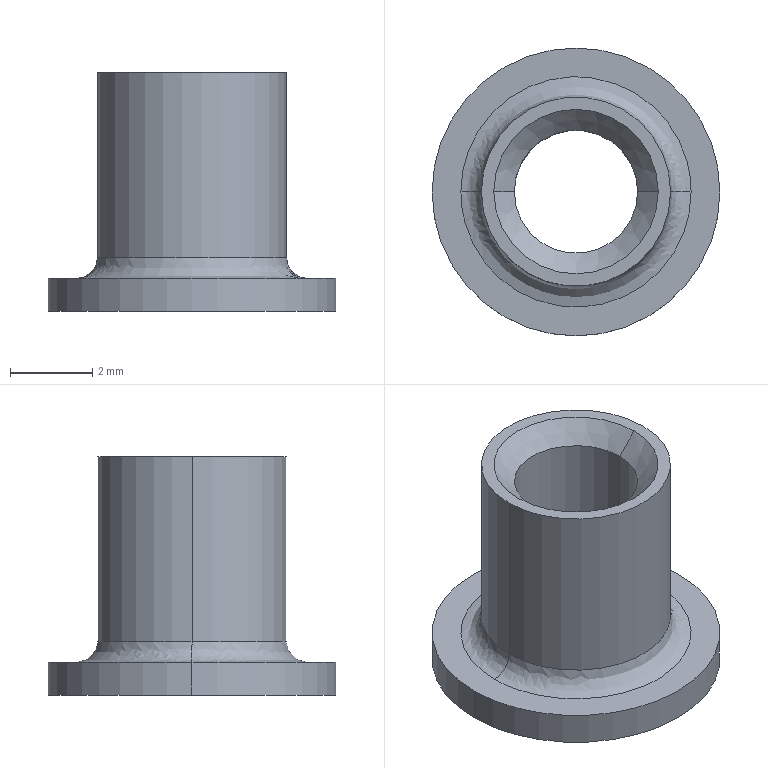Part | SolidWorks | features BaseBody 1 | 1 solid | 13 faces | box 7 x 7 x 5.8 mm | volume 72.379 mm3 | cylinder 6 | plane 3 | spline 2 | cone 2 | commonest cylinder face diameters 3 x2 4.6 x2 7 x2
STEP:
#1=CARTESIAN_POINT('',(-2.8,0.,0.8));
#2=VERTEX_POINT('',#1);
#3=CARTESIAN_POINT('',(2.8,0.,0.8));
#4=VERTEX_POINT('',#3);
#5=CARTESIAN_POINT('',(-2.8,0.,0.8));
#6=CARTESIAN_POINT('',(-2.8,0.1782,0.8));
#7=CARTESIAN_POINT('',(-2.775,0.4407,0.8));
#8=CARTESIAN_POINT('',(-2.704,0.7385,0.8));
#9=CARTESIAN_POINT('',(-2.657,0.8853,0.8));
#10=CARTESIAN_POINT('',(-2.635,0.9477,0.8));
#11=CARTESIAN_POINT('',(-2.62,0.9893,0.8));
#12=CARTESIAN_POINT('',(-2.612,1.008,0.8));
#13=CARTESIAN_POINT('',(-2.461,1.39,0.8));
#14=CARTESIAN_POINT('',(-2.254,1.706,0.8));
#15=CARTESIAN_POINT('',(-1.843,2.117,0.8));
#16=CARTESIAN_POINT('',(-1.622,2.297,0.8));
#17=CARTESIAN_POINT('',(-1.336,2.465,0.8));
#18=CARTESIAN_POINT('',(-1.185,2.538,0.8));
#19=CARTESIAN_POINT('',(-1.12,2.567,0.8));
#20=CARTESIAN_POINT('',(-1.075,2.585,0.8));
#21=CARTESIAN_POINT('',(-1.051,2.595,0.8));
#22=CARTESIAN_POINT('',(-0.6993,2.735,0.8));
#23=CARTESIAN_POINT('',(-0.3564,2.8,0.8));
#24=CARTESIAN_POINT('',(0.1782,2.8,0.8));
#25=CARTESIAN_POINT('',(0.4407,2.775,0.8));
#26=CARTESIAN_POINT('',(0.7385,2.704,0.8));
#27=CARTESIAN_POINT('',(0.8853,2.657,0.8));
#28=CARTESIAN_POINT('',(0.9477,2.635,0.8));
#29=CARTESIAN_POINT('',(0.9893,2.62,0.8));
#30=CARTESIAN_POINT('',(1.008,2.612,0.8));
#31=CARTESIAN_POINT('',(1.39,2.461,0.8));
#32=CARTESIAN_POINT('',(1.706,2.254,0.8));
#33=CARTESIAN_POINT('',(2.117,1.843,0.8));
#34=CARTESIAN_POINT('',(2.297,1.622,0.8));
#35=CARTESIAN_POINT('',(2.465,1.336,0.8));
#36=CARTESIAN_POINT('',(2.538,1.185,0.8));
#37=CARTESIAN_POINT('',(2.567,1.12,0.8));
#38=CARTESIAN_POINT('',(2.585,1.075,0.8));
#39=CARTESIAN_POINT('',(2.595,1.051,0.8));
#40=CARTESIAN_POINT('',(2.734,0.6998,0.8));
#41=CARTESIAN_POINT('',(2.8,0.3562,0.8));
#42=CARTESIAN_POINT('',(2.8,0.,0.8));
#43=B_SPLINE_CURVE_WITH_KNOTS('',3,(#5,#6,#7,#8,#9,#10,#11,#12,#13,#14,#15,#16,#17,#18,#19,#20,#21,#22,#23,#24,#25,#26,#27,#28,#29,#30,#31,#32,#33,#34,#35,#36,#37,#38,#39,#40,#41,#42),.UNSPECIFIED.,.F.,.F.,(4,1,1,1,2,2,2,1,1,1,2,2,2,1,1,1,2,2,2,1,1,1,2,2,4),(0.5,0.5312,0.5469,0.5547,0.5586,0.5625,0.625,0.6562,0.6719,0.6797,0.6836,0.6875,0.75,0.7812,0.7969,0.8047,0.8086,0.8125,0.875,0.9062,0.9219,0.9297,0.9336,0.9375,1.),.UNSPECIFIED.);
#44=EDGE_CURVE('',#2,#4,#43,.T.);
#45=ORIENTED_EDGE('',*,*,#44,.F.);
#46=CARTESIAN_POINT('',(-2.3,0.,1.3));
#47=VERTEX_POINT('',#46);
#48=CARTESIAN_POINT('',(-2.8,0.,1.3));
#49=DIRECTION('',(0.,-1.,0.));
#50=DIRECTION('',(-1.,0.,0.));
#51=AXIS2_PLACEMENT_3D('',#48,#49,#50);
#52=CIRCLE('',#51,0.5);
#53=EDGE_CURVE('',#2,#47,#52,.T.);
#54=ORIENTED_EDGE('',*,*,#53,.T.);
#55=CARTESIAN_POINT('',(2.3,0.,1.3));
#56=VERTEX_POINT('',#55);
#57=CARTESIAN_POINT('',(0.,0.,1.3));
#58=DIRECTION('',(0.,0.,1.));
#59=DIRECTION('',(-1.,0.,0.));
#60=AXIS2_PLACEMENT_3D('',#57,#58,#59);
#61=CIRCLE('',#60,2.3);
#62=EDGE_CURVE('',#56,#47,#61,.T.);
#63=ORIENTED_EDGE('',*,*,#62,.F.);
#64=CARTESIAN_POINT('',(2.8,0.,1.3));
#65=DIRECTION('',(0.,1.,0.));
#66=DIRECTION('',(1.,0.,0.));
#67=AXIS2_PLACEMENT_3D('',#64,#65,#66);
#68=CIRCLE('',#67,0.5);
#69=EDGE_CURVE('',#4,#56,#68,.T.);
#70=ORIENTED_EDGE('',*,*,#69,.F.);
#71=EDGE_LOOP('',(#45,#54,#63,#70));
#72=FACE_OUTER_BOUND('',#71,.T.);
#73=CARTESIAN_POINT('',(2.8,0.,0.8));
#74=CARTESIAN_POINT('',(2.8,5.6,0.8));
#75=CARTESIAN_POINT('',(-2.8,5.6,0.8));
#76=CARTESIAN_POINT('',(-2.8,0.,0.8));
#77=CARTESIAN_POINT('',(2.507,0.,0.8));
#78=CARTESIAN_POINT('',(2.507,5.014,0.8));
#79=CARTESIAN_POINT('',(-2.507,5.014,0.8));
#80=CARTESIAN_POINT('',(-2.507,0.,0.8));
#81=CARTESIAN_POINT('',(2.3,0.,1.007));
#82=CARTESIAN_POINT('',(2.3,4.6,1.007));
#83=CARTESIAN_POINT('',(-2.3,4.6,1.007));
#84=CARTESIAN_POINT('',(-2.3,0.,1.007));
#85=CARTESIAN_POINT('',(2.3,0.,1.3));
#86=CARTESIAN_POINT('',(2.3,4.6,1.3));
#87=CARTESIAN_POINT('',(-2.3,4.6,1.3));
#88=CARTESIAN_POINT('',(-2.3,0.,1.3));
#89=(BOUNDED_SURFACE()B_SPLINE_SURFACE(3,3,((#73,#74,#75,#76),(#77,#78,#79,#80),(#81,#82,#83,#84),(#85,#86,#87,#88)),.UNSPECIFIED.,.F.,.F.,.F.)B_SPLINE_SURFACE_WITH_KNOTS((4,4),(4,4),(0.,1.),(0.,1.),.UNSPECIFIED.)GEOMETRIC_REPRESENTATION_ITEM()RATIONAL_B_SPLINE_SURFACE(((1.,0.3333,0.3333,1.),(0.8047,0.2682,0.2682,0.8047),(0.8047,0.2682,0.2682,0.8047),(1.,0.3333,0.3333,1.)))REPRESENTATION_ITEM('')SURFACE());
#90=ADVANCED_FACE('',(#72),#89,.F.);
#91=CARTESIAN_POINT('',(-2.3,0.,5.8));
#92=VERTEX_POINT('',#91);
#93=CARTESIAN_POINT('',(2.3,0.,5.8));
#94=VERTEX_POINT('',#93);
#95=CARTESIAN_POINT('',(0.,0.,5.8));
#96=DIRECTION('',(0.,0.,-1.));
#97=DIRECTION('',(-1.,0.,0.));
#98=AXIS2_PLACEMENT_3D('',#95,#96,#97);
#99=CIRCLE('',#98,2.3);
#100=EDGE_CURVE('',#92,#94,#99,.T.);
#101=ORIENTED_EDGE('',*,*,#100,.T.);
#102=CARTESIAN_POINT('',(2.3,0.,5.8));
#103=DIRECTION('',(0.,0.,-1.));
#104=VECTOR('',#103,1000.);
#105=LINE('',#102,#104);
#106=EDGE_CURVE('',#94,#56,#105,.T.);
#107=ORIENTED_EDGE('',*,*,#106,.T.);
#108=ORIENTED_EDGE('',*,*,#62,.T.);
#109=CARTESIAN_POINT('',(-2.3,0.,5.8));
#110=DIRECTION('',(0.,0.,-1.));
#111=VECTOR('',#110,1000.);
#112=LINE('',#109,#111);
#113=EDGE_CURVE('',#92,#47,#112,.T.);
#114=ORIENTED_EDGE('',*,*,#113,.F.);
#115=EDGE_LOOP('',(#101,#107,#108,#114));
#116=FACE_OUTER_BOUND('',#115,.T.);
#117=CARTESIAN_POINT('',(0.,0.,5.8));
#118=DIRECTION('',(0.,0.,-1.));
#119=DIRECTION('',(-1.,0.,0.));
#120=AXIS2_PLACEMENT_3D('',#117,#118,#119);
#121=CYLINDRICAL_SURFACE('',#120,2.3);
#122=ADVANCED_FACE('',(#116),#121,.T.);
#123=CARTESIAN_POINT('',(-1.5,0.,5.3));
#124=VERTEX_POINT('',#123);
#125=CARTESIAN_POINT('',(1.5,0.,5.3));
#126=VERTEX_POINT('',#125);
#127=CARTESIAN_POINT('',(0.,0.,5.3));
#128=DIRECTION('',(0.,0.,1.));
#129=DIRECTION('',(-1.,0.,0.));
#130=AXIS2_PLACEMENT_3D('',#127,#128,#129);
#131=CIRCLE('',#130,1.5);
#132=EDGE_CURVE('',#124,#126,#131,.T.);
#133=ORIENTED_EDGE('',*,*,#132,.F.);
#134=CARTESIAN_POINT('',(-2.,0.,5.8));
#135=VERTEX_POINT('',#134);
#136=CARTESIAN_POINT('',(-2.,0.,5.8));
#137=DIRECTION('',(-0.7071,0.,0.7071));
#138=VECTOR('',#137,1000.);
#139=LINE('',#136,#138);
#140=EDGE_CURVE('',#124,#135,#139,.T.);
#141=ORIENTED_EDGE('',*,*,#140,.T.);
#142=CARTESIAN_POINT('',(2.,0.,5.8));
#143=VERTEX_POINT('',#142);
#144=CARTESIAN_POINT('',(0.,0.,5.8));
#145=DIRECTION('',(0.,0.,1.));
#146=DIRECTION('',(1.,0.,0.));
#147=AXIS2_PLACEMENT_3D('',#144,#145,#146);
#148=CIRCLE('',#147,2.);
#149=EDGE_CURVE('',#135,#143,#148,.T.);
#150=ORIENTED_EDGE('',*,*,#149,.T.);
#151=CARTESIAN_POINT('',(2.,0.,5.8));
#152=DIRECTION('',(0.7071,0.,0.7071));
#153=VECTOR('',#152,1000.);
#154=LINE('',#151,#153);
#155=EDGE_CURVE('',#126,#143,#154,.T.);
#156=ORIENTED_EDGE('',*,*,#155,.F.);
#157=EDGE_LOOP('',(#133,#141,#150,#156));
#158=FACE_OUTER_BOUND('',#157,.T.);
#159=CARTESIAN_POINT('',(0.,0.,5.8));
#160=DIRECTION('',(0.,0.,1.));
#161=DIRECTION('',(1.,0.,0.));
#162=AXIS2_PLACEMENT_3D('',#159,#160,#161);
#163=CONICAL_SURFACE('',#162,2.,0.7854);
#164=ADVANCED_FACE('',(#158),#163,.F.);
#165=CARTESIAN_POINT('',(3.5,0.,0.));
#166=VERTEX_POINT('',#165);
#167=CARTESIAN_POINT('',(-3.5,0.,0.));
#168=VERTEX_POINT('',#167);
#169=CARTESIAN_POINT('',(0.,0.,0.));
#170=DIRECTION('',(0.,0.,1.));
#171=DIRECTION('',(1.,0.,0.));
#172=AXIS2_PLACEMENT_3D('',#169,#170,#171);
#173=CIRCLE('',#172,3.5);
#174=EDGE_CURVE('',#166,#168,#173,.T.);
#175=ORIENTED_EDGE('',*,*,#174,.T.);
#176=CARTESIAN_POINT('',(-3.5,0.,0.8));
#177=VERTEX_POINT('',#176);
#178=CARTESIAN_POINT('',(-3.5,0.,0.));
#179=DIRECTION('',(0.,0.,1.));
#180=VECTOR('',#179,1000.);
#181=LINE('',#178,#180);
#182=EDGE_CURVE('',#168,#177,#181,.T.);
#183=ORIENTED_EDGE('',*,*,#182,.T.);
#184=CARTESIAN_POINT('',(3.5,0.,0.8));
#185=VERTEX_POINT('',#184);
#186=CARTESIAN_POINT('',(0.,0.,0.8));
#187=DIRECTION('',(0.,0.,-1.));
#188=DIRECTION('',(1.,0.,0.));
#189=AXIS2_PLACEMENT_3D('',#186,#187,#188);
#190=CIRCLE('',#189,3.5);
#191=EDGE_CURVE('',#177,#185,#190,.T.);
#192=ORIENTED_EDGE('',*,*,#191,.T.);
#193=CARTESIAN_POINT('',(3.5,0.,0.));
#194=DIRECTION('',(0.,0.,1.));
#195=VECTOR('',#194,1000.);
#196=LINE('',#193,#195);
#197=EDGE_CURVE('',#166,#185,#196,.T.);
#198=ORIENTED_EDGE('',*,*,#197,.F.);
#199=EDGE_LOOP('',(#175,#183,#192,#198));
#200=FACE_OUTER_BOUND('',#199,.T.);
#201=CARTESIAN_POINT('',(0.,0.,0.));
#202=DIRECTION('',(0.,0.,1.));
#203=DIRECTION('',(1.,0.,0.));
#204=AXIS2_PLACEMENT_3D('',#201,#202,#203);
#205=CYLINDRICAL_SURFACE('',#204,3.5);
#206=ADVANCED_FACE('',(#200),#205,.T.);
#207=CARTESIAN_POINT('',(-1.5,0.,0.));
#208=VERTEX_POINT('',#207);
#209=CARTESIAN_POINT('',(1.5,0.,0.));
#210=VERTEX_POINT('',#209);
#211=CARTESIAN_POINT('',(0.,0.,0.));
#212=DIRECTION('',(0.,0.,1.));
#213=DIRECTION('',(1.,0.,0.));
#214=AXIS2_PLACEMENT_3D('',#211,#212,#213);
#215=CIRCLE('',#214,1.5);
#216=EDGE_CURVE('',#208,#210,#215,.T.);
#217=ORIENTED_EDGE('',*,*,#216,.F.);
#218=CARTESIAN_POINT('',(-1.5,0.,-5.673));
#219=DIRECTION('',(0.,0.,1.));
#220=VECTOR('',#219,1000.);
#221=LINE('',#218,#220);
#222=EDGE_CURVE('',#208,#124,#221,.T.);
#223=ORIENTED_EDGE('',*,*,#222,.T.);
#224=ORIENTED_EDGE('',*,*,#132,.T.);
#225=CARTESIAN_POINT('',(1.5,0.,-5.673));
#226=DIRECTION('',(0.,0.,1.));
#227=VECTOR('',#226,1000.);
#228=LINE('',#225,#227);
#229=EDGE_CURVE('',#210,#126,#228,.T.);
#230=ORIENTED_EDGE('',*,*,#229,.F.);
#231=EDGE_LOOP('',(#217,#223,#224,#230));
#232=FACE_OUTER_BOUND('',#231,.T.);
#233=CARTESIAN_POINT('',(0.,0.,-5.673));
#234=DIRECTION('',(0.,0.,1.));
#235=DIRECTION('',(1.,0.,0.));
#236=AXIS2_PLACEMENT_3D('',#233,#234,#235);
#237=CYLINDRICAL_SURFACE('',#236,1.5);
#238=ADVANCED_FACE('',(#232),#237,.F.);
#239=ORIENTED_EDGE('',*,*,#106,.F.);
#240=CARTESIAN_POINT('',(0.,0.,5.8));
#241=DIRECTION('',(0.,0.,-1.));
#242=DIRECTION('',(-1.,0.,0.));
#243=AXIS2_PLACEMENT_3D('',#240,#241,#242);
#244=CIRCLE('',#243,2.3);
#245=EDGE_CURVE('',#94,#92,#244,.T.);
#246=ORIENTED_EDGE('',*,*,#245,.T.);
#247=ORIENTED_EDGE('',*,*,#113,.T.);
#248=CARTESIAN_POINT('',(0.,0.,1.3));
#249=DIRECTION('',(0.,0.,1.));
#250=DIRECTION('',(-1.,0.,0.));
#251=AXIS2_PLACEMENT_3D('',#248,#249,#250);
#252=CIRCLE('',#251,2.3);
#253=EDGE_CURVE('',#47,#56,#252,.T.);
#254=ORIENTED_EDGE('',*,*,#253,.T.);
#255=EDGE_LOOP('',(#239,#246,#247,#254));
#256=FACE_OUTER_BOUND('',#255,.T.);
#257=CARTESIAN_POINT('',(0.,0.,5.8));
#258=DIRECTION('',(0.,0.,-1.));
#259=DIRECTION('',(-1.,0.,0.));
#260=AXIS2_PLACEMENT_3D('',#257,#258,#259);
#261=CYLINDRICAL_SURFACE('',#260,2.3);
#262=ADVANCED_FACE('',(#256),#261,.T.);
#263=ORIENTED_EDGE('',*,*,#53,.F.);
#264=CARTESIAN_POINT('',(2.8,0.,0.8));
#265=CARTESIAN_POINT('',(2.8,-0.1779,0.8));
#266=CARTESIAN_POINT('',(2.776,-0.4402,0.8));
#267=CARTESIAN_POINT('',(2.704,-0.7382,0.8));
#268=CARTESIAN_POINT('',(2.657,-0.8851,0.8));
#269=CARTESIAN_POINT('',(2.635,-0.9476,0.8));
#270=CARTESIAN_POINT('',(2.62,-0.9892,0.8));
#271=CARTESIAN_POINT('',(2.612,-1.008,0.8));
#272=CARTESIAN_POINT('',(2.461,-1.39,0.8));
#273=CARTESIAN_POINT('',(2.254,-1.706,0.8));
#274=CARTESIAN_POINT('',(1.843,-2.117,0.8));
#275=CARTESIAN_POINT('',(1.622,-2.297,0.8));
#276=CARTESIAN_POINT('',(1.336,-2.465,0.8));
#277=CARTESIAN_POINT('',(1.185,-2.538,0.8));
#278=CARTESIAN_POINT('',(1.12,-2.567,0.8));
#279=CARTESIAN_POINT('',(1.075,-2.585,0.8));
#280=CARTESIAN_POINT('',(1.051,-2.595,0.8));
#281=CARTESIAN_POINT('',(0.6993,-2.735,0.8));
#282=CARTESIAN_POINT('',(0.3564,-2.8,0.8));
#283=CARTESIAN_POINT('',(-0.1782,-2.8,0.8));
#284=CARTESIAN_POINT('',(-0.4407,-2.775,0.8));
#285=CARTESIAN_POINT('',(-0.7385,-2.704,0.8));
#286=CARTESIAN_POINT('',(-0.8853,-2.657,0.8));
#287=CARTESIAN_POINT('',(-0.9477,-2.635,0.8));
#288=CARTESIAN_POINT('',(-0.9893,-2.62,0.8));
#289=CARTESIAN_POINT('',(-1.008,-2.612,0.8));
#290=CARTESIAN_POINT('',(-1.39,-2.461,0.8));
#291=CARTESIAN_POINT('',(-1.706,-2.254,0.8));
#292=CARTESIAN_POINT('',(-2.117,-1.843,0.8));
#293=CARTESIAN_POINT('',(-2.297,-1.622,0.8));
#294=CARTESIAN_POINT('',(-2.465,-1.336,0.8));
#295=CARTESIAN_POINT('',(-2.538,-1.185,0.8));
#296=CARTESIAN_POINT('',(-2.567,-1.12,0.8));
#297=CARTESIAN_POINT('',(-2.585,-1.075,0.8));
#298=CARTESIAN_POINT('',(-2.595,-1.051,0.8));
#299=CARTESIAN_POINT('',(-2.735,-0.6993,0.8));
#300=CARTESIAN_POINT('',(-2.8,-0.3564,0.8));
#301=CARTESIAN_POINT('',(-2.8,0.,0.8));
#302=B_SPLINE_CURVE_WITH_KNOTS('',3,(#264,#265,#266,#267,#268,#269,#270,#271,#272,#273,#274,#275,#276,#277,#278,#279,#280,#281,#282,#283,#284,#285,#286,#287,#288,#289,#290,#291,#292,#293,#294,#295,#296,#297,#298,#299,#300,#301),.UNSPECIFIED.,.F.,.F.,(4,1,1,1,2,2,2,1,1,1,2,2,2,1,1,1,2,2,2,1,1,1,2,2,4),(0.,0.03125,0.04688,0.05469,0.05859,0.0625,0.125,0.1563,0.1719,0.1797,0.1836,0.1875,0.25,0.2813,0.2969,0.3047,0.3086,0.3125,0.375,0.4062,0.4219,0.4297,0.4336,0.4375,0.5),.UNSPECIFIED.);
#303=EDGE_CURVE('',#4,#2,#302,.T.);
#304=ORIENTED_EDGE('',*,*,#303,.F.);
#305=ORIENTED_EDGE('',*,*,#69,.T.);
#306=ORIENTED_EDGE('',*,*,#253,.F.);
#307=EDGE_LOOP('',(#263,#304,#305,#306));
#308=FACE_OUTER_BOUND('',#307,.T.);
#309=CARTESIAN_POINT('',(-2.8,0.,0.8));
#310=CARTESIAN_POINT('',(-2.8,-5.6,0.8));
#311=CARTESIAN_POINT('',(2.8,-5.6,0.8));
#312=CARTESIAN_POINT('',(2.8,0.,0.8));
#313=CARTESIAN_POINT('',(-2.507,0.,0.8));
#314=CARTESIAN_POINT('',(-2.507,-5.014,0.8));
#315=CARTESIAN_POINT('',(2.507,-5.014,0.8));
#316=CARTESIAN_POINT('',(2.507,0.,0.8));
#317=CARTESIAN_POINT('',(-2.3,0.,1.007));
#318=CARTESIAN_POINT('',(-2.3,-4.6,1.007));
#319=CARTESIAN_POINT('',(2.3,-4.6,1.007));
#320=CARTESIAN_POINT('',(2.3,0.,1.007));
#321=CARTESIAN_POINT('',(-2.3,0.,1.3));
#322=CARTESIAN_POINT('',(-2.3,-4.6,1.3));
#323=CARTESIAN_POINT('',(2.3,-4.6,1.3));
#324=CARTESIAN_POINT('',(2.3,0.,1.3));
#325=(BOUNDED_SURFACE()B_SPLINE_SURFACE(3,3,((#309,#310,#311,#312),(#313,#314,#315,#316),(#317,#318,#319,#320),(#321,#322,#323,#324)),.UNSPECIFIED.,.F.,.F.,.F.)B_SPLINE_SURFACE_WITH_KNOTS((4,4),(4,4),(0.,1.),(0.,1.),.UNSPECIFIED.)GEOMETRIC_REPRESENTATION_ITEM()RATIONAL_B_SPLINE_SURFACE(((1.,0.3333,0.3333,1.),(0.8047,0.2682,0.2682,0.8047),(0.8047,0.2682,0.2682,0.8047),(1.,0.3333,0.3333,1.)))REPRESENTATION_ITEM('')SURFACE());
#326=ADVANCED_FACE('',(#308),#325,.F.);
#327=CARTESIAN_POINT('',(0.,0.,5.8));
#328=DIRECTION('',(0.,0.,1.));
#329=DIRECTION('',(1.,0.,0.));
#330=AXIS2_PLACEMENT_3D('',#327,#328,#329);
#331=CIRCLE('',#330,2.);
#332=EDGE_CURVE('',#143,#135,#331,.T.);
#333=ORIENTED_EDGE('',*,*,#332,.F.);
#334=ORIENTED_EDGE('',*,*,#149,.F.);
#335=EDGE_LOOP('',(#333,#334));
#336=FACE_BOUND('',#335,.T.);
#337=ORIENTED_EDGE('',*,*,#100,.F.);
#338=ORIENTED_EDGE('',*,*,#245,.F.);
#339=EDGE_LOOP('',(#337,#338));
#340=FACE_OUTER_BOUND('',#339,.T.);
#341=CARTESIAN_POINT('',(0.,0.,5.8));
#342=DIRECTION('',(0.,0.,-1.));
#343=DIRECTION('',(-1.,0.,0.));
#344=AXIS2_PLACEMENT_3D('',#341,#342,#343);
#345=PLANE('',#344);
#346=ADVANCED_FACE('',(#336,#340),#345,.F.);
#347=ORIENTED_EDGE('',*,*,#303,.T.);
#348=ORIENTED_EDGE('',*,*,#44,.T.);
#349=EDGE_LOOP('',(#347,#348));
#350=FACE_BOUND('',#349,.T.);
#351=CARTESIAN_POINT('',(0.,0.,0.8));
#352=DIRECTION('',(0.,0.,-1.));
#353=DIRECTION('',(1.,0.,0.));
#354=AXIS2_PLACEMENT_3D('',#351,#352,#353);
#355=CIRCLE('',#354,3.5);
#356=EDGE_CURVE('',#185,#177,#355,.T.);
#357=ORIENTED_EDGE('',*,*,#356,.F.);
#358=ORIENTED_EDGE('',*,*,#191,.F.);
#359=EDGE_LOOP('',(#357,#358));
#360=FACE_OUTER_BOUND('',#359,.T.);
#361=CARTESIAN_POINT('',(0.,0.,0.8));
#362=DIRECTION('',(0.,0.,-1.));
#363=DIRECTION('',(-1.,0.,0.));
#364=AXIS2_PLACEMENT_3D('',#361,#362,#363);
#365=PLANE('',#364);
#366=ADVANCED_FACE('',(#350,#360),#365,.F.);
#367=ORIENTED_EDGE('',*,*,#140,.F.);
#368=CARTESIAN_POINT('',(0.,0.,5.3));
#369=DIRECTION('',(0.,0.,1.));
#370=DIRECTION('',(-1.,0.,0.));
#371=AXIS2_PLACEMENT_3D('',#368,#369,#370);
#372=CIRCLE('',#371,1.5);
#373=EDGE_CURVE('',#126,#124,#372,.T.);
#374=ORIENTED_EDGE('',*,*,#373,.F.);
#375=ORIENTED_EDGE('',*,*,#155,.T.);
#376=ORIENTED_EDGE('',*,*,#332,.T.);
#377=EDGE_LOOP('',(#367,#374,#375,#376));
#378=FACE_OUTER_BOUND('',#377,.T.);
#379=CARTESIAN_POINT('',(0.,0.,5.8));
#380=DIRECTION('',(0.,0.,1.));
#381=DIRECTION('',(1.,0.,0.));
#382=AXIS2_PLACEMENT_3D('',#379,#380,#381);
#383=CONICAL_SURFACE('',#382,2.,0.7854);
#384=ADVANCED_FACE('',(#378),#383,.F.);
#385=ORIENTED_EDGE('',*,*,#182,.F.);
#386=CARTESIAN_POINT('',(0.,0.,0.));
#387=DIRECTION('',(0.,0.,1.));
#388=DIRECTION('',(1.,0.,0.));
#389=AXIS2_PLACEMENT_3D('',#386,#387,#388);
#390=CIRCLE('',#389,3.5);
#391=EDGE_CURVE('',#168,#166,#390,.T.);
#392=ORIENTED_EDGE('',*,*,#391,.T.);
#393=ORIENTED_EDGE('',*,*,#197,.T.);
#394=ORIENTED_EDGE('',*,*,#356,.T.);
#395=EDGE_LOOP('',(#385,#392,#393,#394));
#396=FACE_OUTER_BOUND('',#395,.T.);
#397=CARTESIAN_POINT('',(0.,0.,0.));
#398=DIRECTION('',(0.,0.,1.));
#399=DIRECTION('',(1.,0.,0.));
#400=AXIS2_PLACEMENT_3D('',#397,#398,#399);
#401=CYLINDRICAL_SURFACE('',#400,3.5);
#402=ADVANCED_FACE('',(#396),#401,.T.);
#403=ORIENTED_EDGE('',*,*,#222,.F.);
#404=CARTESIAN_POINT('',(0.,0.,0.));
#405=DIRECTION('',(0.,0.,1.));
#406=DIRECTION('',(1.,0.,0.));
#407=AXIS2_PLACEMENT_3D('',#404,#405,#406);
#408=CIRCLE('',#407,1.5);
#409=EDGE_CURVE('',#210,#208,#408,.T.);
#410=ORIENTED_EDGE('',*,*,#409,.F.);
#411=ORIENTED_EDGE('',*,*,#229,.T.);
#412=ORIENTED_EDGE('',*,*,#373,.T.);
#413=EDGE_LOOP('',(#403,#410,#411,#412));
#414=FACE_OUTER_BOUND('',#413,.T.);
#415=CARTESIAN_POINT('',(0.,0.,-5.673));
#416=DIRECTION('',(0.,0.,1.));
#417=DIRECTION('',(1.,0.,0.));
#418=AXIS2_PLACEMENT_3D('',#415,#416,#417);
#419=CYLINDRICAL_SURFACE('',#418,1.5);
#420=ADVANCED_FACE('',(#414),#419,.F.);
#421=ORIENTED_EDGE('',*,*,#409,.T.);
#422=ORIENTED_EDGE('',*,*,#216,.T.);
#423=EDGE_LOOP('',(#421,#422));
#424=FACE_BOUND('',#423,.T.);
#425=ORIENTED_EDGE('',*,*,#174,.F.);
#426=ORIENTED_EDGE('',*,*,#391,.F.);
#427=EDGE_LOOP('',(#425,#426));
#428=FACE_OUTER_BOUND('',#427,.T.);
#429=CARTESIAN_POINT('',(0.,0.,0.));
#430=DIRECTION('',(0.,0.,-1.));
#431=DIRECTION('',(-1.,0.,0.));
#432=AXIS2_PLACEMENT_3D('',#429,#430,#431);
#433=PLANE('',#432);
#434=ADVANCED_FACE('',(#424,#428),#433,.T.);
#435=CLOSED_SHELL('',(#90,#122,#164,#206,#238,#262,#326,#346,#366,#384,#402,#420,#434));
#436=MANIFOLD_SOLID_BREP('',#435);
#437=CARTESIAN_POINT('',(0.,0.,0.));
#438=DIRECTION('',(0.,0.,1.));
#439=DIRECTION('',(1.,0.,0.));
#440=AXIS2_PLACEMENT_3D('',#437,#438,#439);
#441=(LENGTH_UNIT()NAMED_UNIT(*)SI_UNIT(.MILLI.,.METRE.));
#442=UNCERTAINTY_MEASURE_WITH_UNIT(LENGTH_MEASURE(0.00001),#441,'','');
#443=(NAMED_UNIT(*)PLANE_ANGLE_UNIT()SI_UNIT($,.RADIAN.));
#444=(NAMED_UNIT(*)SI_UNIT($,.STERADIAN.)SOLID_ANGLE_UNIT());
#445=(GEOMETRIC_REPRESENTATION_CONTEXT(3)GLOBAL_UNCERTAINTY_ASSIGNED_CONTEXT((#442))GLOBAL_UNIT_ASSIGNED_CONTEXT((#441,#443,#444))REPRESENTATION_CONTEXT('',''));
#446=ADVANCED_BREP_SHAPE_REPRESENTATION('',(#436,#440),#445);